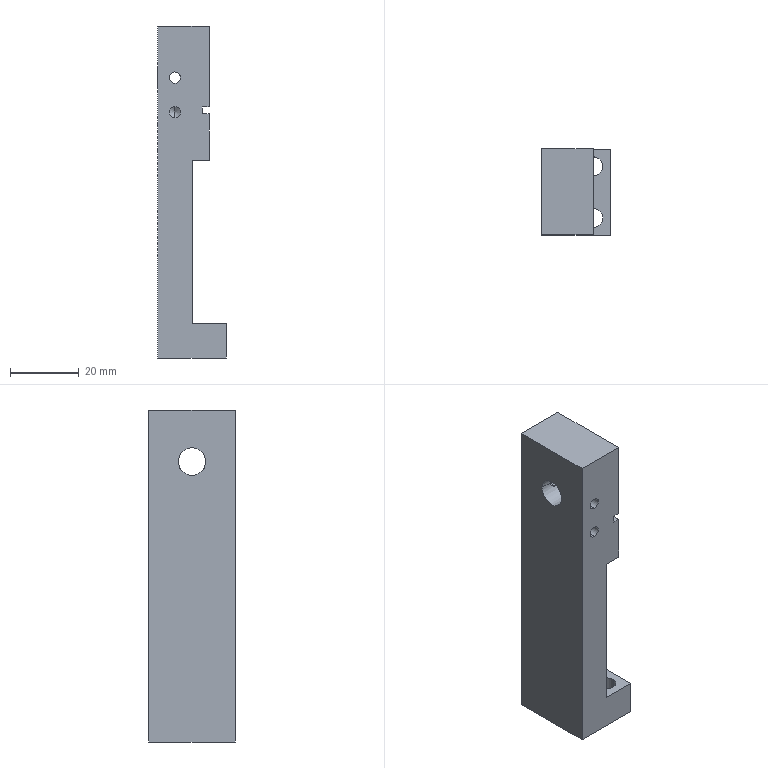Part | STEP file | 11-FG-B00211 | 1 solid | 40 faces | box 20 x 25 x 96.4 mm | volume 29627 mm3 | cylinder 18 | plane 14 | cone 8 | commonest cylinder face diameters 3.3 x12 5.5 x4 8 x2
STEP:
#1=CARTESIAN_POINT('',(4.,5.,71.65));
#2=VERTEX_POINT('',#1);
#3=CARTESIAN_POINT('',(4.,5.,68.35));
#4=VERTEX_POINT('',#3);
#5=CARTESIAN_POINT('',(4.,5.,70.));
#6=DIRECTION('',(1.,0.,0.));
#7=DIRECTION('',(0.,0.,-1.));
#8=AXIS2_PLACEMENT_3D('',#5,#6,#7);
#9=CIRCLE('',#8,1.65);
#10=EDGE_CURVE('',#2,#4,#9,.T.);
#11=ORIENTED_EDGE('',*,*,#10,.F.);
#12=CARTESIAN_POINT('',(15.,5.,71.65));
#13=VERTEX_POINT('',#12);
#14=CARTESIAN_POINT('',(15.,5.,71.65));
#15=DIRECTION('',(1.,0.,0.));
#16=VECTOR('',#15,1000.);
#17=LINE('',#14,#16);
#18=EDGE_CURVE('',#2,#13,#17,.T.);
#19=ORIENTED_EDGE('',*,*,#18,.T.);
#20=CARTESIAN_POINT('',(15.,5.,68.35));
#21=VERTEX_POINT('',#20);
#22=CARTESIAN_POINT('',(15.,5.,70.));
#23=DIRECTION('',(1.,0.,0.));
#24=DIRECTION('',(0.,0.,-1.));
#25=AXIS2_PLACEMENT_3D('',#22,#23,#24);
#26=CIRCLE('',#25,1.65);
#27=EDGE_CURVE('',#13,#21,#26,.T.);
#28=ORIENTED_EDGE('',*,*,#27,.T.);
#29=CARTESIAN_POINT('',(15.,5.,68.35));
#30=DIRECTION('',(1.,0.,0.));
#31=VECTOR('',#30,1000.);
#32=LINE('',#29,#31);
#33=EDGE_CURVE('',#4,#21,#32,.T.);
#34=ORIENTED_EDGE('',*,*,#33,.F.);
#35=EDGE_LOOP('',(#11,#19,#28,#34));
#36=FACE_OUTER_BOUND('',#35,.T.);
#37=CARTESIAN_POINT('',(15.,5.,70.));
#38=DIRECTION('',(1.,0.,0.));
#39=DIRECTION('',(0.,0.,-1.));
#40=AXIS2_PLACEMENT_3D('',#37,#38,#39);
#41=CYLINDRICAL_SURFACE('',#40,1.65);
#42=ADVANCED_FACE('',(#36),#41,.F.);
#43=CARTESIAN_POINT('',(3.009,5.,70.));
#44=VERTEX_POINT('',#43);
#45=CARTESIAN_POINT('',(4.,5.,68.35));
#46=DIRECTION('',(0.515,0.,-0.8572));
#47=VECTOR('',#46,1000.);
#48=LINE('',#45,#47);
#49=EDGE_CURVE('',#44,#4,#48,.T.);
#50=ORIENTED_EDGE('',*,*,#49,.F.);
#51=CARTESIAN_POINT('',(4.,5.,71.65));
#52=DIRECTION('',(0.515,0.,0.8572));
#53=VECTOR('',#52,1000.);
#54=LINE('',#51,#53);
#55=EDGE_CURVE('',#44,#2,#54,.T.);
#56=ORIENTED_EDGE('',*,*,#55,.T.);
#57=ORIENTED_EDGE('',*,*,#10,.T.);
#58=EDGE_LOOP('',(#50,#56,#57));
#59=FACE_OUTER_BOUND('',#58,.T.);
#60=CARTESIAN_POINT('',(4.,5.,70.));
#61=DIRECTION('',(1.,0.,0.));
#62=DIRECTION('',(0.,0.,-1.));
#63=AXIS2_PLACEMENT_3D('',#60,#61,#62);
#64=CONICAL_SURFACE('',#63,1.65,1.03);
#65=ADVANCED_FACE('',(#59),#64,.F.);
#66=CARTESIAN_POINT('',(4.,20.,71.65));
#67=VERTEX_POINT('',#66);
#68=CARTESIAN_POINT('',(4.,20.,68.35));
#69=VERTEX_POINT('',#68);
#70=CARTESIAN_POINT('',(4.,20.,70.));
#71=DIRECTION('',(1.,0.,0.));
#72=DIRECTION('',(0.,0.,-1.));
#73=AXIS2_PLACEMENT_3D('',#70,#71,#72);
#74=CIRCLE('',#73,1.65);
#75=EDGE_CURVE('',#67,#69,#74,.T.);
#76=ORIENTED_EDGE('',*,*,#75,.F.);
#77=CARTESIAN_POINT('',(15.,20.,71.65));
#78=VERTEX_POINT('',#77);
#79=CARTESIAN_POINT('',(15.,20.,71.65));
#80=DIRECTION('',(1.,0.,0.));
#81=VECTOR('',#80,1000.);
#82=LINE('',#79,#81);
#83=EDGE_CURVE('',#67,#78,#82,.T.);
#84=ORIENTED_EDGE('',*,*,#83,.T.);
#85=CARTESIAN_POINT('',(15.,20.,68.35));
#86=VERTEX_POINT('',#85);
#87=CARTESIAN_POINT('',(15.,20.,70.));
#88=DIRECTION('',(1.,0.,0.));
#89=DIRECTION('',(0.,0.,-1.));
#90=AXIS2_PLACEMENT_3D('',#87,#88,#89);
#91=CIRCLE('',#90,1.65);
#92=EDGE_CURVE('',#78,#86,#91,.T.);
#93=ORIENTED_EDGE('',*,*,#92,.T.);
#94=CARTESIAN_POINT('',(15.,20.,68.35));
#95=DIRECTION('',(1.,0.,0.));
#96=VECTOR('',#95,1000.);
#97=LINE('',#94,#96);
#98=EDGE_CURVE('',#69,#86,#97,.T.);
#99=ORIENTED_EDGE('',*,*,#98,.F.);
#100=EDGE_LOOP('',(#76,#84,#93,#99));
#101=FACE_OUTER_BOUND('',#100,.T.);
#102=CARTESIAN_POINT('',(15.,20.,70.));
#103=DIRECTION('',(1.,0.,0.));
#104=DIRECTION('',(0.,0.,-1.));
#105=AXIS2_PLACEMENT_3D('',#102,#103,#104);
#106=CYLINDRICAL_SURFACE('',#105,1.65);
#107=ADVANCED_FACE('',(#101),#106,.F.);
#108=CARTESIAN_POINT('',(3.009,20.,70.));
#109=VERTEX_POINT('',#108);
#110=CARTESIAN_POINT('',(4.,20.,68.35));
#111=DIRECTION('',(0.515,0.,-0.8572));
#112=VECTOR('',#111,1000.);
#113=LINE('',#110,#112);
#114=EDGE_CURVE('',#109,#69,#113,.T.);
#115=ORIENTED_EDGE('',*,*,#114,.F.);
#116=CARTESIAN_POINT('',(4.,20.,71.65));
#117=DIRECTION('',(0.515,0.,0.8572));
#118=VECTOR('',#117,1000.);
#119=LINE('',#116,#118);
#120=EDGE_CURVE('',#109,#67,#119,.T.);
#121=ORIENTED_EDGE('',*,*,#120,.T.);
#122=ORIENTED_EDGE('',*,*,#75,.T.);
#123=EDGE_LOOP('',(#115,#121,#122));
#124=FACE_OUTER_BOUND('',#123,.T.);
#125=CARTESIAN_POINT('',(4.,20.,70.));
#126=DIRECTION('',(1.,0.,0.));
#127=DIRECTION('',(0.,0.,-1.));
#128=AXIS2_PLACEMENT_3D('',#125,#126,#127);
#129=CONICAL_SURFACE('',#128,1.65,1.03);
#130=ADVANCED_FACE('',(#124),#129,.F.);
#131=CARTESIAN_POINT('',(5.,10.1,65.65));
#132=VERTEX_POINT('',#131);
#133=CARTESIAN_POINT('',(5.,10.1,62.35));
#134=VERTEX_POINT('',#133);
#135=CARTESIAN_POINT('',(5.,10.1,64.));
#136=DIRECTION('',(0.,-1.,0.));
#137=DIRECTION('',(0.,0.,-1.));
#138=AXIS2_PLACEMENT_3D('',#135,#136,#137);
#139=CIRCLE('',#138,1.65);
#140=EDGE_CURVE('',#132,#134,#139,.T.);
#141=ORIENTED_EDGE('',*,*,#140,.F.);
#142=CARTESIAN_POINT('',(5.,0.,65.65));
#143=VERTEX_POINT('',#142);
#144=CARTESIAN_POINT('',(5.,0.,65.65));
#145=DIRECTION('',(0.,-1.,0.));
#146=VECTOR('',#145,1000.);
#147=LINE('',#144,#146);
#148=EDGE_CURVE('',#132,#143,#147,.T.);
#149=ORIENTED_EDGE('',*,*,#148,.T.);
#150=CARTESIAN_POINT('',(5.,0.,62.35));
#151=VERTEX_POINT('',#150);
#152=CARTESIAN_POINT('',(5.,0.,64.));
#153=DIRECTION('',(0.,-1.,0.));
#154=DIRECTION('',(0.,0.,-1.));
#155=AXIS2_PLACEMENT_3D('',#152,#153,#154);
#156=CIRCLE('',#155,1.65);
#157=EDGE_CURVE('',#143,#151,#156,.T.);
#158=ORIENTED_EDGE('',*,*,#157,.T.);
#159=CARTESIAN_POINT('',(5.,0.,62.35));
#160=DIRECTION('',(0.,-1.,0.));
#161=VECTOR('',#160,1000.);
#162=LINE('',#159,#161);
#163=EDGE_CURVE('',#134,#151,#162,.T.);
#164=ORIENTED_EDGE('',*,*,#163,.F.);
#165=EDGE_LOOP('',(#141,#149,#158,#164));
#166=FACE_OUTER_BOUND('',#165,.T.);
#167=CARTESIAN_POINT('',(5.,0.,64.));
#168=DIRECTION('',(0.,-1.,0.));
#169=DIRECTION('',(0.,0.,-1.));
#170=AXIS2_PLACEMENT_3D('',#167,#168,#169);
#171=CYLINDRICAL_SURFACE('',#170,1.65);
#172=ADVANCED_FACE('',(#166),#171,.F.);
#173=CARTESIAN_POINT('',(5.,11.091,64.));
#174=VERTEX_POINT('',#173);
#175=CARTESIAN_POINT('',(5.,10.1,62.35));
#176=DIRECTION('',(0.,-0.515,-0.8572));
#177=VECTOR('',#176,1000.);
#178=LINE('',#175,#177);
#179=EDGE_CURVE('',#174,#134,#178,.T.);
#180=ORIENTED_EDGE('',*,*,#179,.F.);
#181=CARTESIAN_POINT('',(5.,10.1,65.65));
#182=DIRECTION('',(0.,-0.515,0.8572));
#183=VECTOR('',#182,1000.);
#184=LINE('',#181,#183);
#185=EDGE_CURVE('',#174,#132,#184,.T.);
#186=ORIENTED_EDGE('',*,*,#185,.T.);
#187=ORIENTED_EDGE('',*,*,#140,.T.);
#188=EDGE_LOOP('',(#180,#186,#187));
#189=FACE_OUTER_BOUND('',#188,.T.);
#190=CARTESIAN_POINT('',(5.,10.1,64.));
#191=DIRECTION('',(0.,-1.,0.));
#192=DIRECTION('',(0.,0.,-1.));
#193=AXIS2_PLACEMENT_3D('',#190,#191,#192);
#194=CONICAL_SURFACE('',#193,1.65,1.03);
#195=ADVANCED_FACE('',(#189),#194,.F.);
#196=CARTESIAN_POINT('',(5.,8.856,75.65));
#197=VERTEX_POINT('',#196);
#198=CARTESIAN_POINT('',(3.35,8.5,74.));
#199=VERTEX_POINT('',#198);
#200=CARTESIAN_POINT('',(5.,8.856,75.65));
#201=CARTESIAN_POINT('',(4.891,8.856,75.65));
#202=CARTESIAN_POINT('',(4.78,8.851,75.639));
#203=CARTESIAN_POINT('',(4.568,8.832,75.596));
#204=CARTESIAN_POINT('',(4.464,8.818,75.564));
#205=CARTESIAN_POINT('',(4.263,8.784,75.48));
#206=CARTESIAN_POINT('',(4.169,8.764,75.429));
#207=CARTESIAN_POINT('',(3.992,8.72,75.31));
#208=CARTESIAN_POINT('',(3.908,8.697,75.241));
#209=CARTESIAN_POINT('',(3.757,8.651,75.091));
#210=CARTESIAN_POINT('',(3.69,8.628,75.008));
#211=CARTESIAN_POINT('',(3.57,8.586,74.83));
#212=CARTESIAN_POINT('',(3.518,8.567,74.734));
#213=CARTESIAN_POINT('',(3.394,8.519,74.437));
#214=CARTESIAN_POINT('',(3.35,8.5,74.217));
#215=CARTESIAN_POINT('',(3.35,8.5,74.));
#216=B_SPLINE_CURVE_WITH_KNOTS('',3,(#200,#201,#202,#203,#204,#205,#206,#207,#208,#209,#210,#211,#212,#213,#214,#215),.UNSPECIFIED.,.F.,.F.,(4,2,2,2,2,2,2,4),(0.00261,0.002936,0.003262,0.003588,0.003914,0.00424,0.004566,0.005218),.UNSPECIFIED.);
#217=EDGE_CURVE('',#197,#199,#216,.T.);
#218=ORIENTED_EDGE('',*,*,#217,.F.);
#219=CARTESIAN_POINT('',(5.,0.,75.65));
#220=VERTEX_POINT('',#219);
#221=CARTESIAN_POINT('',(5.,0.,75.65));
#222=DIRECTION('',(0.,-1.,0.));
#223=VECTOR('',#222,1000.);
#224=LINE('',#221,#223);
#225=EDGE_CURVE('',#197,#220,#224,.T.);
#226=ORIENTED_EDGE('',*,*,#225,.T.);
#227=CARTESIAN_POINT('',(5.,0.,72.35));
#228=VERTEX_POINT('',#227);
#229=CARTESIAN_POINT('',(5.,0.,74.));
#230=DIRECTION('',(0.,-1.,0.));
#231=DIRECTION('',(0.,0.,-1.));
#232=AXIS2_PLACEMENT_3D('',#229,#230,#231);
#233=CIRCLE('',#232,1.65);
#234=EDGE_CURVE('',#220,#228,#233,.T.);
#235=ORIENTED_EDGE('',*,*,#234,.T.);
#236=CARTESIAN_POINT('',(5.,8.856,72.35));
#237=VERTEX_POINT('',#236);
#238=CARTESIAN_POINT('',(5.,0.,72.35));
#239=DIRECTION('',(0.,-1.,0.));
#240=VECTOR('',#239,1000.);
#241=LINE('',#238,#240);
#242=EDGE_CURVE('',#237,#228,#241,.T.);
#243=ORIENTED_EDGE('',*,*,#242,.F.);
#244=CARTESIAN_POINT('',(3.35,8.5,74.));
#245=CARTESIAN_POINT('',(3.35,8.5,73.891));
#246=CARTESIAN_POINT('',(3.361,8.505,73.781));
#247=CARTESIAN_POINT('',(3.404,8.522,73.567));
#248=CARTESIAN_POINT('',(3.436,8.535,73.464));
#249=CARTESIAN_POINT('',(3.561,8.583,73.164));
#250=CARTESIAN_POINT('',(3.682,8.628,72.984));
#251=CARTESIAN_POINT('',(3.91,8.697,72.756));
#252=CARTESIAN_POINT('',(3.993,8.72,72.689));
#253=CARTESIAN_POINT('',(4.17,8.764,72.57));
#254=CARTESIAN_POINT('',(4.266,8.784,72.518));
#255=CARTESIAN_POINT('',(4.465,8.818,72.435));
#256=CARTESIAN_POINT('',(4.568,8.832,72.404));
#257=CARTESIAN_POINT('',(4.781,8.851,72.361));
#258=CARTESIAN_POINT('',(4.891,8.856,72.35));
#259=CARTESIAN_POINT('',(5.,8.856,72.35));
#260=B_SPLINE_CURVE_WITH_KNOTS('',3,(#244,#245,#246,#247,#248,#249,#250,#251,#252,#253,#254,#255,#256,#257,#258,#259),.UNSPECIFIED.,.F.,.F.,(4,2,2,2,2,2,2,4),(0.005218,0.005543,0.005869,0.006521,0.006847,0.007173,0.007499,0.007825),.UNSPECIFIED.);
#261=EDGE_CURVE('',#199,#237,#260,.T.);
#262=ORIENTED_EDGE('',*,*,#261,.F.);
#263=EDGE_LOOP('',(#218,#226,#235,#243,#262));
#264=FACE_OUTER_BOUND('',#263,.T.);
#265=CARTESIAN_POINT('',(5.,0.,74.));
#266=DIRECTION('',(0.,-1.,0.));
#267=DIRECTION('',(0.,0.,-1.));
#268=AXIS2_PLACEMENT_3D('',#265,#266,#267);
#269=CYLINDRICAL_SURFACE('',#268,1.65);
#270=ADVANCED_FACE('',(#264),#269,.F.);
#271=CARTESIAN_POINT('',(12.25,5.,-7.4));
#272=VERTEX_POINT('',#271);
#273=CARTESIAN_POINT('',(17.75,5.,-7.4));
#274=VERTEX_POINT('',#273);
#275=CARTESIAN_POINT('',(15.,5.,-7.4));
#276=DIRECTION('',(0.,0.,1.));
#277=DIRECTION('',(1.,0.,0.));
#278=AXIS2_PLACEMENT_3D('',#275,#276,#277);
#279=CIRCLE('',#278,2.75);
#280=EDGE_CURVE('',#272,#274,#279,.T.);
#281=ORIENTED_EDGE('',*,*,#280,.F.);
#282=CARTESIAN_POINT('',(12.25,5.,2.6));
#283=VERTEX_POINT('',#282);
#284=CARTESIAN_POINT('',(12.25,5.,0.));
#285=DIRECTION('',(0.,0.,1.));
#286=VECTOR('',#285,1000.);
#287=LINE('',#284,#286);
#288=EDGE_CURVE('',#272,#283,#287,.T.);
#289=ORIENTED_EDGE('',*,*,#288,.T.);
#290=CARTESIAN_POINT('',(17.75,5.,2.6));
#291=VERTEX_POINT('',#290);
#292=CARTESIAN_POINT('',(15.,5.,2.6));
#293=DIRECTION('',(0.,0.,1.));
#294=DIRECTION('',(1.,0.,0.));
#295=AXIS2_PLACEMENT_3D('',#292,#293,#294);
#296=CIRCLE('',#295,2.75);
#297=EDGE_CURVE('',#283,#291,#296,.T.);
#298=ORIENTED_EDGE('',*,*,#297,.T.);
#299=CARTESIAN_POINT('',(17.75,5.,0.));
#300=DIRECTION('',(0.,0.,1.));
#301=VECTOR('',#300,1000.);
#302=LINE('',#299,#301);
#303=EDGE_CURVE('',#274,#291,#302,.T.);
#304=ORIENTED_EDGE('',*,*,#303,.F.);
#305=EDGE_LOOP('',(#281,#289,#298,#304));
#306=FACE_OUTER_BOUND('',#305,.T.);
#307=CARTESIAN_POINT('',(15.,5.,0.));
#308=DIRECTION('',(0.,0.,1.));
#309=DIRECTION('',(1.,0.,0.));
#310=AXIS2_PLACEMENT_3D('',#307,#308,#309);
#311=CYLINDRICAL_SURFACE('',#310,2.75);
#312=ADVANCED_FACE('',(#306),#311,.F.);
#313=CARTESIAN_POINT('',(12.25,20.,-7.4));
#314=VERTEX_POINT('',#313);
#315=CARTESIAN_POINT('',(17.75,20.,-7.4));
#316=VERTEX_POINT('',#315);
#317=CARTESIAN_POINT('',(15.,20.,-7.4));
#318=DIRECTION('',(0.,0.,1.));
#319=DIRECTION('',(1.,0.,0.));
#320=AXIS2_PLACEMENT_3D('',#317,#318,#319);
#321=CIRCLE('',#320,2.75);
#322=EDGE_CURVE('',#314,#316,#321,.T.);
#323=ORIENTED_EDGE('',*,*,#322,.F.);
#324=CARTESIAN_POINT('',(12.25,20.,2.6));
#325=VERTEX_POINT('',#324);
#326=CARTESIAN_POINT('',(12.25,20.,0.));
#327=DIRECTION('',(0.,0.,1.));
#328=VECTOR('',#327,1000.);
#329=LINE('',#326,#328);
#330=EDGE_CURVE('',#314,#325,#329,.T.);
#331=ORIENTED_EDGE('',*,*,#330,.T.);
#332=CARTESIAN_POINT('',(17.75,20.,2.6));
#333=VERTEX_POINT('',#332);
#334=CARTESIAN_POINT('',(15.,20.,2.6));
#335=DIRECTION('',(0.,0.,1.));
#336=DIRECTION('',(1.,0.,0.));
#337=AXIS2_PLACEMENT_3D('',#334,#335,#336);
#338=CIRCLE('',#337,2.75);
#339=EDGE_CURVE('',#325,#333,#338,.T.);
#340=ORIENTED_EDGE('',*,*,#339,.T.);
#341=CARTESIAN_POINT('',(17.75,20.,0.));
#342=DIRECTION('',(0.,0.,1.));
#343=VECTOR('',#342,1000.);
#344=LINE('',#341,#343);
#345=EDGE_CURVE('',#316,#333,#344,.T.);
#346=ORIENTED_EDGE('',*,*,#345,.F.);
#347=EDGE_LOOP('',(#323,#331,#340,#346));
#348=FACE_OUTER_BOUND('',#347,.T.);
#349=CARTESIAN_POINT('',(15.,20.,0.));
#350=DIRECTION('',(0.,0.,1.));
#351=DIRECTION('',(1.,0.,0.));
#352=AXIS2_PLACEMENT_3D('',#349,#350,#351);
#353=CYLINDRICAL_SURFACE('',#352,2.75);
#354=ADVANCED_FACE('',(#348),#353,.F.);
#355=CARTESIAN_POINT('',(5.,16.144,72.35));
#356=VERTEX_POINT('',#355);
#357=CARTESIAN_POINT('',(3.35,16.5,74.));
#358=VERTEX_POINT('',#357);
#359=CARTESIAN_POINT('',(5.,16.144,72.35));
#360=CARTESIAN_POINT('',(4.891,16.144,72.35));
#361=CARTESIAN_POINT('',(4.781,16.149,72.361));
#362=CARTESIAN_POINT('',(4.568,16.168,72.404));
#363=CARTESIAN_POINT('',(4.464,16.182,72.436));
#364=CARTESIAN_POINT('',(4.165,16.233,72.561));
#365=CARTESIAN_POINT('',(3.985,16.28,72.682));
#366=CARTESIAN_POINT('',(3.757,16.349,72.91));
#367=CARTESIAN_POINT('',(3.689,16.372,72.992));
#368=CARTESIAN_POINT('',(3.571,16.414,73.169));
#369=CARTESIAN_POINT('',(3.519,16.433,73.265));
#370=CARTESIAN_POINT('',(3.436,16.465,73.465));
#371=CARTESIAN_POINT('',(3.404,16.478,73.568));
#372=CARTESIAN_POINT('',(3.361,16.495,73.781));
#373=CARTESIAN_POINT('',(3.35,16.5,73.891));
#374=CARTESIAN_POINT('',(3.35,16.5,74.));
#375=B_SPLINE_CURVE_WITH_KNOTS('',3,(#359,#360,#361,#362,#363,#364,#365,#366,#367,#368,#369,#370,#371,#372,#373,#374),.UNSPECIFIED.,.F.,.F.,(4,2,2,2,2,2,2,4),(0.005217,0.005543,0.005869,0.006521,0.006847,0.007172,0.007498,0.007824),.UNSPECIFIED.);
#376=EDGE_CURVE('',#356,#358,#375,.T.);
#377=ORIENTED_EDGE('',*,*,#376,.F.);
#378=CARTESIAN_POINT('',(5.,25.,72.35));
#379=VERTEX_POINT('',#378);
#380=CARTESIAN_POINT('',(5.,25.,72.35));
#381=DIRECTION('',(0.,1.,0.));
#382=VECTOR('',#381,1000.);
#383=LINE('',#380,#382);
#384=EDGE_CURVE('',#356,#379,#383,.T.);
#385=ORIENTED_EDGE('',*,*,#384,.T.);
#386=CARTESIAN_POINT('',(5.,25.,75.65));
#387=VERTEX_POINT('',#386);
#388=CARTESIAN_POINT('',(5.,25.,74.));
#389=DIRECTION('',(0.,1.,0.));
#390=DIRECTION('',(0.,0.,1.));
#391=AXIS2_PLACEMENT_3D('',#388,#389,#390);
#392=CIRCLE('',#391,1.65);
#393=EDGE_CURVE('',#379,#387,#392,.T.);
#394=ORIENTED_EDGE('',*,*,#393,.T.);
#395=CARTESIAN_POINT('',(5.,16.144,75.65));
#396=VERTEX_POINT('',#395);
#397=CARTESIAN_POINT('',(5.,25.,75.65));
#398=DIRECTION('',(0.,1.,0.));
#399=VECTOR('',#398,1000.);
#400=LINE('',#397,#399);
#401=EDGE_CURVE('',#396,#387,#400,.T.);
#402=ORIENTED_EDGE('',*,*,#401,.F.);
#403=CARTESIAN_POINT('',(3.35,16.5,74.));
#404=CARTESIAN_POINT('',(3.35,16.5,74.218));
#405=CARTESIAN_POINT('',(3.394,16.481,74.437));
#406=CARTESIAN_POINT('',(3.519,16.433,74.735));
#407=CARTESIAN_POINT('',(3.571,16.414,74.831));
#408=CARTESIAN_POINT('',(3.69,16.372,75.009));
#409=CARTESIAN_POINT('',(3.758,16.349,75.091));
#410=CARTESIAN_POINT('',(3.909,16.303,75.243));
#411=CARTESIAN_POINT('',(3.993,16.279,75.311));
#412=CARTESIAN_POINT('',(4.17,16.236,75.43));
#413=CARTESIAN_POINT('',(4.264,16.216,75.481));
#414=CARTESIAN_POINT('',(4.565,16.164,75.607));
#415=CARTESIAN_POINT('',(4.779,16.144,75.65));
#416=CARTESIAN_POINT('',(5.,16.144,75.65));
#417=B_SPLINE_CURVE_WITH_KNOTS('',3,(#403,#404,#405,#406,#407,#408,#409,#410,#411,#412,#413,#414,#415,#416),.UNSPECIFIED.,.F.,.F.,(4,2,2,2,2,2,4),(0.007824,0.008476,0.008802,0.009127,0.009453,0.009779,0.01043),.UNSPECIFIED.);
#418=EDGE_CURVE('',#358,#396,#417,.T.);
#419=ORIENTED_EDGE('',*,*,#418,.F.);
#420=EDGE_LOOP('',(#377,#385,#394,#402,#419));
#421=FACE_OUTER_BOUND('',#420,.T.);
#422=CARTESIAN_POINT('',(5.,25.,74.));
#423=DIRECTION('',(0.,1.,0.));
#424=DIRECTION('',(0.,0.,1.));
#425=AXIS2_PLACEMENT_3D('',#422,#423,#424);
#426=CYLINDRICAL_SURFACE('',#425,1.65);
#427=ADVANCED_FACE('',(#421),#426,.F.);
#428=CARTESIAN_POINT('',(5.,14.9,62.35));
#429=VERTEX_POINT('',#428);
#430=CARTESIAN_POINT('',(5.,14.9,65.65));
#431=VERTEX_POINT('',#430);
#432=CARTESIAN_POINT('',(5.,14.9,64.));
#433=DIRECTION('',(0.,1.,0.));
#434=DIRECTION('',(0.,0.,1.));
#435=AXIS2_PLACEMENT_3D('',#432,#433,#434);
#436=CIRCLE('',#435,1.65);
#437=EDGE_CURVE('',#429,#431,#436,.T.);
#438=ORIENTED_EDGE('',*,*,#437,.F.);
#439=CARTESIAN_POINT('',(5.,25.,62.35));
#440=VERTEX_POINT('',#439);
#441=CARTESIAN_POINT('',(5.,25.,62.35));
#442=DIRECTION('',(0.,1.,0.));
#443=VECTOR('',#442,1000.);
#444=LINE('',#441,#443);
#445=EDGE_CURVE('',#429,#440,#444,.T.);
#446=ORIENTED_EDGE('',*,*,#445,.T.);
#447=CARTESIAN_POINT('',(5.,25.,65.65));
#448=VERTEX_POINT('',#447);
#449=CARTESIAN_POINT('',(5.,25.,64.));
#450=DIRECTION('',(0.,1.,0.));
#451=DIRECTION('',(0.,0.,1.));
#452=AXIS2_PLACEMENT_3D('',#449,#450,#451);
#453=CIRCLE('',#452,1.65);
#454=EDGE_CURVE('',#440,#448,#453,.T.);
#455=ORIENTED_EDGE('',*,*,#454,.T.);
#456=CARTESIAN_POINT('',(5.,25.,65.65));
#457=DIRECTION('',(0.,1.,0.));
#458=VECTOR('',#457,1000.);
#459=LINE('',#456,#458);
#460=EDGE_CURVE('',#431,#448,#459,.T.);
#461=ORIENTED_EDGE('',*,*,#460,.F.);
#462=EDGE_LOOP('',(#438,#446,#455,#461));
#463=FACE_OUTER_BOUND('',#462,.T.);
#464=CARTESIAN_POINT('',(5.,25.,64.));
#465=DIRECTION('',(0.,1.,0.));
#466=DIRECTION('',(0.,0.,1.));
#467=AXIS2_PLACEMENT_3D('',#464,#465,#466);
#468=CYLINDRICAL_SURFACE('',#467,1.65);
#469=ADVANCED_FACE('',(#463),#468,.F.);
#470=CARTESIAN_POINT('',(5.,13.909,64.));
#471=VERTEX_POINT('',#470);
#472=CARTESIAN_POINT('',(5.,14.9,65.65));
#473=DIRECTION('',(0.,0.515,0.8572));
#474=VECTOR('',#473,1000.);
#475=LINE('',#472,#474);
#476=EDGE_CURVE('',#471,#431,#475,.T.);
#477=ORIENTED_EDGE('',*,*,#476,.F.);
#478=CARTESIAN_POINT('',(5.,14.9,62.35));
#479=DIRECTION('',(0.,0.515,-0.8572));
#480=VECTOR('',#479,1000.);
#481=LINE('',#478,#480);
#482=EDGE_CURVE('',#471,#429,#481,.T.);
#483=ORIENTED_EDGE('',*,*,#482,.T.);
#484=ORIENTED_EDGE('',*,*,#437,.T.);
#485=EDGE_LOOP('',(#477,#483,#484));
#486=FACE_OUTER_BOUND('',#485,.T.);
#487=CARTESIAN_POINT('',(5.,14.9,64.));
#488=DIRECTION('',(0.,1.,0.));
#489=DIRECTION('',(0.,0.,1.));
#490=AXIS2_PLACEMENT_3D('',#487,#488,#489);
#491=CONICAL_SURFACE('',#490,1.65,1.03);
#492=ADVANCED_FACE('',(#486),#491,.F.);
#493=CARTESIAN_POINT('',(15.,16.5,74.));
#494=VERTEX_POINT('',#493);
#495=CARTESIAN_POINT('',(15.,8.5,74.));
#496=VERTEX_POINT('',#495);
#497=CARTESIAN_POINT('',(15.,12.5,74.));
#498=DIRECTION('',(-1.,0.,0.));
#499=DIRECTION('',(0.,-1.,0.));
#500=AXIS2_PLACEMENT_3D('',#497,#498,#499);
#501=CIRCLE('',#500,4.);
#502=EDGE_CURVE('',#494,#496,#501,.T.);
#503=ORIENTED_EDGE('',*,*,#502,.F.);
#504=CARTESIAN_POINT('',(6.65,16.5,74.));
#505=VERTEX_POINT('',#504);
#506=CARTESIAN_POINT('',(20.,16.5,74.));
#507=DIRECTION('',(-1.,0.,0.));
#508=VECTOR('',#507,1000.);
#509=LINE('',#506,#508);
#510=EDGE_CURVE('',#494,#505,#509,.T.);
#511=ORIENTED_EDGE('',*,*,#510,.T.);
#512=CARTESIAN_POINT('',(6.65,16.5,74.));
#513=CARTESIAN_POINT('',(6.65,16.5,73.891));
#514=CARTESIAN_POINT('',(6.639,16.495,73.78));
#515=CARTESIAN_POINT('',(6.596,16.478,73.568));
#516=CARTESIAN_POINT('',(6.564,16.465,73.464));
#517=CARTESIAN_POINT('',(6.48,16.433,73.263));
#518=CARTESIAN_POINT('',(6.429,16.414,73.168));
#519=CARTESIAN_POINT('',(6.31,16.372,72.991));
#520=CARTESIAN_POINT('',(6.241,16.349,72.907));
#521=CARTESIAN_POINT('',(6.09,16.303,72.756));
#522=CARTESIAN_POINT('',(6.008,16.28,72.689));
#523=CARTESIAN_POINT('',(5.829,16.236,72.57));
#524=CARTESIAN_POINT('',(5.734,16.216,72.518));
#525=CARTESIAN_POINT('',(5.437,16.165,72.394));
#526=CARTESIAN_POINT('',(5.217,16.144,72.35));
#527=CARTESIAN_POINT('',(5.,16.144,72.35));
#528=B_SPLINE_CURVE_WITH_KNOTS('',3,(#512,#513,#514,#515,#516,#517,#518,#519,#520,#521,#522,#523,#524,#525,#526,#527),.UNSPECIFIED.,.F.,.F.,(4,2,2,2,2,2,2,4),(0.00261,0.002935,0.003261,0.003587,0.003913,0.004239,0.004565,0.005217),.UNSPECIFIED.);
#529=EDGE_CURVE('',#505,#356,#528,.T.);
#530=ORIENTED_EDGE('',*,*,#529,.T.);
#531=ORIENTED_EDGE('',*,*,#376,.T.);
#532=CARTESIAN_POINT('',(0.,16.5,74.));
#533=VERTEX_POINT('',#532);
#534=CARTESIAN_POINT('',(20.,16.5,74.));
#535=DIRECTION('',(-1.,0.,0.));
#536=VECTOR('',#535,1000.);
#537=LINE('',#534,#536);
#538=EDGE_CURVE('',#358,#533,#537,.T.);
#539=ORIENTED_EDGE('',*,*,#538,.T.);
#540=CARTESIAN_POINT('',(0.,8.5,74.));
#541=VERTEX_POINT('',#540);
#542=CARTESIAN_POINT('',(0.,12.5,74.));
#543=DIRECTION('',(-1.,0.,0.));
#544=DIRECTION('',(0.,-1.,0.));
#545=AXIS2_PLACEMENT_3D('',#542,#543,#544);
#546=CIRCLE('',#545,4.);
#547=EDGE_CURVE('',#533,#541,#546,.T.);
#548=ORIENTED_EDGE('',*,*,#547,.T.);
#549=CARTESIAN_POINT('',(20.,8.5,74.));
#550=DIRECTION('',(-1.,0.,0.));
#551=VECTOR('',#550,1000.);
#552=LINE('',#549,#551);
#553=EDGE_CURVE('',#199,#541,#552,.T.);
#554=ORIENTED_EDGE('',*,*,#553,.F.);
#555=ORIENTED_EDGE('',*,*,#261,.T.);
#556=CARTESIAN_POINT('',(6.65,8.5,74.));
#557=VERTEX_POINT('',#556);
#558=CARTESIAN_POINT('',(5.,8.856,72.35));
#559=CARTESIAN_POINT('',(5.217,8.856,72.35));
#560=CARTESIAN_POINT('',(5.436,8.835,72.394));
#561=CARTESIAN_POINT('',(5.734,8.784,72.519));
#562=CARTESIAN_POINT('',(5.831,8.764,72.57));
#563=CARTESIAN_POINT('',(6.008,8.72,72.69));
#564=CARTESIAN_POINT('',(6.09,8.697,72.757));
#565=CARTESIAN_POINT('',(6.242,8.651,72.908));
#566=CARTESIAN_POINT('',(6.311,8.628,72.992));
#567=CARTESIAN_POINT('',(6.429,8.586,73.169));
#568=CARTESIAN_POINT('',(6.48,8.567,73.263));
#569=CARTESIAN_POINT('',(6.607,8.518,73.565));
#570=CARTESIAN_POINT('',(6.65,8.5,73.78));
#571=CARTESIAN_POINT('',(6.65,8.5,74.));
#572=B_SPLINE_CURVE_WITH_KNOTS('',3,(#558,#559,#560,#561,#562,#563,#564,#565,#566,#567,#568,#569,#570,#571),.UNSPECIFIED.,.F.,.F.,(4,2,2,2,2,2,4),(0.007825,0.008476,0.008802,0.009128,0.009454,0.00978,0.01043),.UNSPECIFIED.);
#573=EDGE_CURVE('',#237,#557,#572,.T.);
#574=ORIENTED_EDGE('',*,*,#573,.T.);
#575=CARTESIAN_POINT('',(20.,8.5,74.));
#576=DIRECTION('',(-1.,0.,0.));
#577=VECTOR('',#576,1000.);
#578=LINE('',#575,#577);
#579=EDGE_CURVE('',#496,#557,#578,.T.);
#580=ORIENTED_EDGE('',*,*,#579,.F.);
#581=EDGE_LOOP('',(#503,#511,#530,#531,#539,#548,#554,#555,#574,#580));
#582=FACE_OUTER_BOUND('',#581,.T.);
#583=CARTESIAN_POINT('',(20.,12.5,74.));
#584=DIRECTION('',(-1.,0.,0.));
#585=DIRECTION('',(0.,-1.,0.));
#586=AXIS2_PLACEMENT_3D('',#583,#584,#585);
#587=CYLINDRICAL_SURFACE('',#586,4.);
#588=ADVANCED_FACE('',(#582),#587,.F.);
#589=CARTESIAN_POINT('',(15.,12.5,74.));
#590=DIRECTION('',(-1.,0.,0.));
#591=DIRECTION('',(0.,-1.,0.));
#592=AXIS2_PLACEMENT_3D('',#589,#590,#591);
#593=CIRCLE('',#592,4.);
#594=EDGE_CURVE('',#496,#494,#593,.T.);
#595=ORIENTED_EDGE('',*,*,#594,.T.);
#596=ORIENTED_EDGE('',*,*,#502,.T.);
#597=EDGE_LOOP('',(#595,#596));
#598=FACE_BOUND('',#597,.T.);
#599=CARTESIAN_POINT('',(15.,20.,70.));
#600=DIRECTION('',(1.,0.,0.));
#601=DIRECTION('',(0.,0.,-1.));
#602=AXIS2_PLACEMENT_3D('',#599,#600,#601);
#603=CIRCLE('',#602,1.65);
#604=EDGE_CURVE('',#86,#78,#603,.T.);
#605=ORIENTED_EDGE('',*,*,#604,.F.);
#606=ORIENTED_EDGE('',*,*,#92,.F.);
#607=EDGE_LOOP('',(#605,#606));
#608=FACE_BOUND('',#607,.T.);
#609=CARTESIAN_POINT('',(15.,5.,70.));
#610=DIRECTION('',(1.,0.,0.));
#611=DIRECTION('',(0.,0.,-1.));
#612=AXIS2_PLACEMENT_3D('',#609,#610,#611);
#613=CIRCLE('',#612,1.65);
#614=EDGE_CURVE('',#21,#13,#613,.T.);
#615=ORIENTED_EDGE('',*,*,#614,.F.);
#616=ORIENTED_EDGE('',*,*,#27,.F.);
#617=EDGE_LOOP('',(#615,#616));
#618=FACE_BOUND('',#617,.T.);
#619=CARTESIAN_POINT('',(15.,0.,89.));
#620=VERTEX_POINT('',#619);
#621=CARTESIAN_POINT('',(15.,0.,65.5));
#622=VERTEX_POINT('',#621);
#623=CARTESIAN_POINT('',(15.,0.,89.));
#624=DIRECTION('',(0.,0.,-1.));
#625=VECTOR('',#624,1000.);
#626=LINE('',#623,#625);
#627=EDGE_CURVE('',#620,#622,#626,.T.);
#628=ORIENTED_EDGE('',*,*,#627,.T.);
#629=CARTESIAN_POINT('',(15.,25.,65.5));
#630=VERTEX_POINT('',#629);
#631=CARTESIAN_POINT('',(15.,-22.,65.5));
#632=DIRECTION('',(0.,1.,0.));
#633=VECTOR('',#632,1000.);
#634=LINE('',#631,#633);
#635=EDGE_CURVE('',#622,#630,#634,.T.);
#636=ORIENTED_EDGE('',*,*,#635,.T.);
#637=CARTESIAN_POINT('',(15.,25.,89.));
#638=VERTEX_POINT('',#637);
#639=CARTESIAN_POINT('',(15.,25.,89.));
#640=DIRECTION('',(0.,0.,-1.));
#641=VECTOR('',#640,1000.);
#642=LINE('',#639,#641);
#643=EDGE_CURVE('',#638,#630,#642,.T.);
#644=ORIENTED_EDGE('',*,*,#643,.F.);
#645=CARTESIAN_POINT('',(15.,0.,89.));
#646=DIRECTION('',(0.,1.,0.));
#647=VECTOR('',#646,1000.);
#648=LINE('',#645,#647);
#649=EDGE_CURVE('',#620,#638,#648,.T.);
#650=ORIENTED_EDGE('',*,*,#649,.F.);
#651=EDGE_LOOP('',(#628,#636,#644,#650));
#652=FACE_OUTER_BOUND('',#651,.T.);
#653=CARTESIAN_POINT('',(15.,0.,89.));
#654=DIRECTION('',(-1.,0.,0.));
#655=DIRECTION('',(0.,-1.,0.));
#656=AXIS2_PLACEMENT_3D('',#653,#654,#655);
#657=PLANE('',#656);
#658=ADVANCED_FACE('',(#598,#608,#618,#652),#657,.F.);
#659=CARTESIAN_POINT('',(0.,12.5,74.));
#660=DIRECTION('',(-1.,0.,0.));
#661=DIRECTION('',(0.,-1.,0.));
#662=AXIS2_PLACEMENT_3D('',#659,#660,#661);
#663=CIRCLE('',#662,4.);
#664=EDGE_CURVE('',#541,#533,#663,.T.);
#665=ORIENTED_EDGE('',*,*,#664,.F.);
#666=ORIENTED_EDGE('',*,*,#547,.F.);
#667=EDGE_LOOP('',(#665,#666));
#668=FACE_BOUND('',#667,.T.);
#669=CARTESIAN_POINT('',(0.,25.,-7.4));
#670=VERTEX_POINT('',#669);
#671=CARTESIAN_POINT('',(0.,0.,-7.4));
#672=VERTEX_POINT('',#671);
#673=CARTESIAN_POINT('',(0.,0.,-7.4));
#674=DIRECTION('',(0.,-1.,0.));
#675=VECTOR('',#674,1000.);
#676=LINE('',#673,#675);
#677=EDGE_CURVE('',#670,#672,#676,.T.);
#678=ORIENTED_EDGE('',*,*,#677,.T.);
#679=CARTESIAN_POINT('',(0.,0.,89.));
#680=VERTEX_POINT('',#679);
#681=CARTESIAN_POINT('',(0.,0.,89.));
#682=DIRECTION('',(0.,0.,-1.));
#683=VECTOR('',#682,1000.);
#684=LINE('',#681,#683);
#685=EDGE_CURVE('',#680,#672,#684,.T.);
#686=ORIENTED_EDGE('',*,*,#685,.F.);
#687=CARTESIAN_POINT('',(0.,25.,89.));
#688=VERTEX_POINT('',#687);
#689=CARTESIAN_POINT('',(0.,0.,89.));
#690=DIRECTION('',(0.,-1.,0.));
#691=VECTOR('',#690,1000.);
#692=LINE('',#689,#691);
#693=EDGE_CURVE('',#688,#680,#692,.T.);
#694=ORIENTED_EDGE('',*,*,#693,.F.);
#695=CARTESIAN_POINT('',(0.,25.,89.));
#696=DIRECTION('',(0.,0.,-1.));
#697=VECTOR('',#696,1000.);
#698=LINE('',#695,#697);
#699=EDGE_CURVE('',#688,#670,#698,.T.);
#700=ORIENTED_EDGE('',*,*,#699,.T.);
#701=EDGE_LOOP('',(#678,#686,#694,#700));
#702=FACE_OUTER_BOUND('',#701,.T.);
#703=CARTESIAN_POINT('',(0.,0.,89.));
#704=DIRECTION('',(1.,0.,0.));
#705=DIRECTION('',(0.,1.,0.));
#706=AXIS2_PLACEMENT_3D('',#703,#704,#705);
#707=PLANE('',#706);
#708=ADVANCED_FACE('',(#668,#702),#707,.F.);
#709=CARTESIAN_POINT('',(5.,0.,64.));
#710=DIRECTION('',(0.,-1.,0.));
#711=DIRECTION('',(0.,0.,-1.));
#712=AXIS2_PLACEMENT_3D('',#709,#710,#711);
#713=CIRCLE('',#712,1.65);
#714=EDGE_CURVE('',#151,#143,#713,.T.);
#715=ORIENTED_EDGE('',*,*,#714,.F.);
#716=ORIENTED_EDGE('',*,*,#157,.F.);
#717=EDGE_LOOP('',(#715,#716));
#718=FACE_BOUND('',#717,.T.);
#719=CARTESIAN_POINT('',(5.,0.,74.));
#720=DIRECTION('',(0.,-1.,0.));
#721=DIRECTION('',(0.,0.,-1.));
#722=AXIS2_PLACEMENT_3D('',#719,#720,#721);
#723=CIRCLE('',#722,1.65);
#724=EDGE_CURVE('',#228,#220,#723,.T.);
#725=ORIENTED_EDGE('',*,*,#724,.F.);
#726=ORIENTED_EDGE('',*,*,#234,.F.);
#727=EDGE_LOOP('',(#725,#726));
#728=FACE_BOUND('',#727,.T.);
#729=CARTESIAN_POINT('',(13.,0.,63.5));
#730=VERTEX_POINT('',#729);
#731=CARTESIAN_POINT('',(13.,0.,65.5));
#732=VERTEX_POINT('',#731);
#733=CARTESIAN_POINT('',(13.,0.,89.));
#734=DIRECTION('',(0.,0.,1.));
#735=VECTOR('',#734,1000.);
#736=LINE('',#733,#735);
#737=EDGE_CURVE('',#730,#732,#736,.T.);
#738=ORIENTED_EDGE('',*,*,#737,.T.);
#739=CARTESIAN_POINT('',(0.,0.,65.5));
#740=DIRECTION('',(1.,0.,0.));
#741=VECTOR('',#740,1000.);
#742=LINE('',#739,#741);
#743=EDGE_CURVE('',#732,#622,#742,.T.);
#744=ORIENTED_EDGE('',*,*,#743,.T.);
#745=ORIENTED_EDGE('',*,*,#627,.F.);
#746=CARTESIAN_POINT('',(0.,0.,89.));
#747=DIRECTION('',(1.,0.,0.));
#748=VECTOR('',#747,1000.);
#749=LINE('',#746,#748);
#750=EDGE_CURVE('',#680,#620,#749,.T.);
#751=ORIENTED_EDGE('',*,*,#750,.F.);
#752=ORIENTED_EDGE('',*,*,#685,.T.);
#753=CARTESIAN_POINT('',(20.,0.,-7.4));
#754=VERTEX_POINT('',#753);
#755=CARTESIAN_POINT('',(0.,0.,-7.4));
#756=DIRECTION('',(1.,0.,0.));
#757=VECTOR('',#756,1000.);
#758=LINE('',#755,#757);
#759=EDGE_CURVE('',#672,#754,#758,.T.);
#760=ORIENTED_EDGE('',*,*,#759,.T.);
#761=CARTESIAN_POINT('',(20.,0.,2.6));
#762=VERTEX_POINT('',#761);
#763=CARTESIAN_POINT('',(20.,0.,10.));
#764=DIRECTION('',(0.,0.,-1.));
#765=VECTOR('',#764,1000.);
#766=LINE('',#763,#765);
#767=EDGE_CURVE('',#762,#754,#766,.T.);
#768=ORIENTED_EDGE('',*,*,#767,.F.);
#769=CARTESIAN_POINT('',(10.,0.,2.6));
#770=VERTEX_POINT('',#769);
#771=CARTESIAN_POINT('',(15.,0.,2.6));
#772=DIRECTION('',(1.,0.,0.));
#773=VECTOR('',#772,1000.);
#774=LINE('',#771,#773);
#775=EDGE_CURVE('',#770,#762,#774,.T.);
#776=ORIENTED_EDGE('',*,*,#775,.F.);
#777=CARTESIAN_POINT('',(10.,0.,50.));
#778=VERTEX_POINT('',#777);
#779=CARTESIAN_POINT('',(10.,0.,10.));
#780=DIRECTION('',(0.,0.,-1.));
#781=VECTOR('',#780,1000.);
#782=LINE('',#779,#781);
#783=EDGE_CURVE('',#778,#770,#782,.T.);
#784=ORIENTED_EDGE('',*,*,#783,.F.);
#785=CARTESIAN_POINT('',(15.,0.,50.));
#786=VERTEX_POINT('',#785);
#787=CARTESIAN_POINT('',(15.,0.,50.));
#788=DIRECTION('',(-1.,0.,0.));
#789=VECTOR('',#788,1000.);
#790=LINE('',#787,#789);
#791=EDGE_CURVE('',#786,#778,#790,.T.);
#792=ORIENTED_EDGE('',*,*,#791,.F.);
#793=CARTESIAN_POINT('',(15.,0.,63.5));
#794=VERTEX_POINT('',#793);
#795=CARTESIAN_POINT('',(15.,0.,89.));
#796=DIRECTION('',(0.,0.,-1.));
#797=VECTOR('',#796,1000.);
#798=LINE('',#795,#797);
#799=EDGE_CURVE('',#794,#786,#798,.T.);
#800=ORIENTED_EDGE('',*,*,#799,.F.);
#801=CARTESIAN_POINT('',(0.,0.,63.5));
#802=DIRECTION('',(-1.,0.,0.));
#803=VECTOR('',#802,1000.);
#804=LINE('',#801,#803);
#805=EDGE_CURVE('',#794,#730,#804,.T.);
#806=ORIENTED_EDGE('',*,*,#805,.T.);
#807=EDGE_LOOP('',(#738,#744,#745,#751,#752,#760,#768,#776,#784,#792,#800,#806));
#808=FACE_OUTER_BOUND('',#807,.T.);
#809=CARTESIAN_POINT('',(0.,0.,89.));
#810=DIRECTION('',(0.,1.,0.));
#811=DIRECTION('',(0.,0.,1.));
#812=AXIS2_PLACEMENT_3D('',#809,#810,#811);
#813=PLANE('',#812);
#814=ADVANCED_FACE('',(#718,#728,#808),#813,.F.);
#815=CARTESIAN_POINT('',(15.,25.,63.5));
#816=VERTEX_POINT('',#815);
#817=CARTESIAN_POINT('',(15.,25.,50.));
#818=VERTEX_POINT('',#817);
#819=CARTESIAN_POINT('',(15.,25.,89.));
#820=DIRECTION('',(0.,0.,-1.));
#821=VECTOR('',#820,1000.);
#822=LINE('',#819,#821);
#823=EDGE_CURVE('',#816,#818,#822,.T.);
#824=ORIENTED_EDGE('',*,*,#823,.F.);
#825=CARTESIAN_POINT('',(15.,-22.,63.5));
#826=DIRECTION('',(0.,1.,0.));
#827=VECTOR('',#826,1000.);
#828=LINE('',#825,#827);
#829=EDGE_CURVE('',#794,#816,#828,.T.);
#830=ORIENTED_EDGE('',*,*,#829,.F.);
#831=ORIENTED_EDGE('',*,*,#799,.T.);
#832=CARTESIAN_POINT('',(15.,72.,50.));
#833=DIRECTION('',(0.,-1.,0.));
#834=VECTOR('',#833,1000.);
#835=LINE('',#832,#834);
#836=EDGE_CURVE('',#818,#786,#835,.T.);
#837=ORIENTED_EDGE('',*,*,#836,.F.);
#838=EDGE_LOOP('',(#824,#830,#831,#837));
#839=FACE_OUTER_BOUND('',#838,.T.);
#840=CARTESIAN_POINT('',(15.,0.,89.));
#841=DIRECTION('',(-1.,0.,0.));
#842=DIRECTION('',(0.,-1.,0.));
#843=AXIS2_PLACEMENT_3D('',#840,#841,#842);
#844=PLANE('',#843);
#845=ADVANCED_FACE('',(#839),#844,.F.);
#846=CARTESIAN_POINT('',(5.,25.,74.));
#847=DIRECTION('',(0.,1.,0.));
#848=DIRECTION('',(0.,0.,1.));
#849=AXIS2_PLACEMENT_3D('',#846,#847,#848);
#850=CIRCLE('',#849,1.65);
#851=EDGE_CURVE('',#387,#379,#850,.T.);
#852=ORIENTED_EDGE('',*,*,#851,.F.);
#853=ORIENTED_EDGE('',*,*,#393,.F.);
#854=EDGE_LOOP('',(#852,#853));
#855=FACE_BOUND('',#854,.T.);
#856=CARTESIAN_POINT('',(5.,25.,64.));
#857=DIRECTION('',(0.,1.,0.));
#858=DIRECTION('',(0.,0.,1.));
#859=AXIS2_PLACEMENT_3D('',#856,#857,#858);
#860=CIRCLE('',#859,1.65);
#861=EDGE_CURVE('',#448,#440,#860,.T.);
#862=ORIENTED_EDGE('',*,*,#861,.F.);
#863=ORIENTED_EDGE('',*,*,#454,.F.);
#864=EDGE_LOOP('',(#862,#863));
#865=FACE_BOUND('',#864,.T.);
#866=ORIENTED_EDGE('',*,*,#643,.T.);
#867=CARTESIAN_POINT('',(13.,25.,65.5));
#868=VERTEX_POINT('',#867);
#869=CARTESIAN_POINT('',(15.,25.,65.5));
#870=DIRECTION('',(1.,0.,0.));
#871=VECTOR('',#870,1000.);
#872=LINE('',#869,#871);
#873=EDGE_CURVE('',#868,#630,#872,.T.);
#874=ORIENTED_EDGE('',*,*,#873,.F.);
#875=CARTESIAN_POINT('',(13.,25.,63.5));
#876=VERTEX_POINT('',#875);
#877=CARTESIAN_POINT('',(13.,25.,65.5));
#878=DIRECTION('',(0.,0.,1.));
#879=VECTOR('',#878,1000.);
#880=LINE('',#877,#879);
#881=EDGE_CURVE('',#876,#868,#880,.T.);
#882=ORIENTED_EDGE('',*,*,#881,.F.);
#883=CARTESIAN_POINT('',(15.,25.,63.5));
#884=DIRECTION('',(-1.,0.,0.));
#885=VECTOR('',#884,1000.);
#886=LINE('',#883,#885);
#887=EDGE_CURVE('',#816,#876,#886,.T.);
#888=ORIENTED_EDGE('',*,*,#887,.F.);
#889=ORIENTED_EDGE('',*,*,#823,.T.);
#890=CARTESIAN_POINT('',(10.,25.,50.));
#891=VERTEX_POINT('',#890);
#892=CARTESIAN_POINT('',(0.,25.,50.));
#893=DIRECTION('',(-1.,0.,0.));
#894=VECTOR('',#893,1000.);
#895=LINE('',#892,#894);
#896=EDGE_CURVE('',#818,#891,#895,.T.);
#897=ORIENTED_EDGE('',*,*,#896,.T.);
#898=CARTESIAN_POINT('',(10.,25.,2.6));
#899=VERTEX_POINT('',#898);
#900=CARTESIAN_POINT('',(10.,25.,89.));
#901=DIRECTION('',(0.,0.,-1.));
#902=VECTOR('',#901,1000.);
#903=LINE('',#900,#902);
#904=EDGE_CURVE('',#891,#899,#903,.T.);
#905=ORIENTED_EDGE('',*,*,#904,.T.);
#906=CARTESIAN_POINT('',(20.,25.,2.6));
#907=VERTEX_POINT('',#906);
#908=CARTESIAN_POINT('',(0.,25.,2.6));
#909=DIRECTION('',(1.,0.,0.));
#910=VECTOR('',#909,1000.);
#911=LINE('',#908,#910);
#912=EDGE_CURVE('',#899,#907,#911,.T.);
#913=ORIENTED_EDGE('',*,*,#912,.T.);
#914=CARTESIAN_POINT('',(20.,25.,-7.4));
#915=VERTEX_POINT('',#914);
#916=CARTESIAN_POINT('',(20.,25.,0.));
#917=DIRECTION('',(0.,0.,1.));
#918=VECTOR('',#917,1000.);
#919=LINE('',#916,#918);
#920=EDGE_CURVE('',#915,#907,#919,.T.);
#921=ORIENTED_EDGE('',*,*,#920,.F.);
#922=CARTESIAN_POINT('',(0.,25.,-7.4));
#923=DIRECTION('',(-1.,0.,0.));
#924=VECTOR('',#923,1000.);
#925=LINE('',#922,#924);
#926=EDGE_CURVE('',#915,#670,#925,.T.);
#927=ORIENTED_EDGE('',*,*,#926,.T.);
#928=ORIENTED_EDGE('',*,*,#699,.F.);
#929=CARTESIAN_POINT('',(0.,25.,89.));
#930=DIRECTION('',(-1.,0.,0.));
#931=VECTOR('',#930,1000.);
#932=LINE('',#929,#931);
#933=EDGE_CURVE('',#638,#688,#932,.T.);
#934=ORIENTED_EDGE('',*,*,#933,.F.);
#935=EDGE_LOOP('',(#866,#874,#882,#888,#889,#897,#905,#913,#921,#927,#928,#934));
#936=FACE_OUTER_BOUND('',#935,.T.);
#937=CARTESIAN_POINT('',(0.,25.,89.));
#938=DIRECTION('',(0.,-1.,0.));
#939=DIRECTION('',(0.,0.,-1.));
#940=AXIS2_PLACEMENT_3D('',#937,#938,#939);
#941=PLANE('',#940);
#942=ADVANCED_FACE('',(#855,#865,#936),#941,.F.);
#943=ORIENTED_EDGE('',*,*,#693,.T.);
#944=ORIENTED_EDGE('',*,*,#750,.T.);
#945=ORIENTED_EDGE('',*,*,#649,.T.);
#946=ORIENTED_EDGE('',*,*,#933,.T.);
#947=EDGE_LOOP('',(#943,#944,#945,#946));
#948=FACE_OUTER_BOUND('',#947,.T.);
#949=CARTESIAN_POINT('',(0.,25.,89.));
#950=DIRECTION('',(0.,0.,-1.));
#951=DIRECTION('',(-1.,0.,0.));
#952=AXIS2_PLACEMENT_3D('',#949,#950,#951);
#953=PLANE('',#952);
#954=ADVANCED_FACE('',(#948),#953,.F.);
#955=CARTESIAN_POINT('',(15.,5.,-7.4));
#956=DIRECTION('',(0.,0.,1.));
#957=DIRECTION('',(1.,0.,0.));
#958=AXIS2_PLACEMENT_3D('',#955,#956,#957);
#959=CIRCLE('',#958,2.75);
#960=EDGE_CURVE('',#274,#272,#959,.T.);
#961=ORIENTED_EDGE('',*,*,#960,.T.);
#962=ORIENTED_EDGE('',*,*,#280,.T.);
#963=EDGE_LOOP('',(#961,#962));
#964=FACE_BOUND('',#963,.T.);
#965=CARTESIAN_POINT('',(15.,20.,-7.4));
#966=DIRECTION('',(0.,0.,1.));
#967=DIRECTION('',(1.,0.,0.));
#968=AXIS2_PLACEMENT_3D('',#965,#966,#967);
#969=CIRCLE('',#968,2.75);
#970=EDGE_CURVE('',#316,#314,#969,.T.);
#971=ORIENTED_EDGE('',*,*,#970,.T.);
#972=ORIENTED_EDGE('',*,*,#322,.T.);
#973=EDGE_LOOP('',(#971,#972));
#974=FACE_BOUND('',#973,.T.);
#975=ORIENTED_EDGE('',*,*,#677,.F.);
#976=ORIENTED_EDGE('',*,*,#926,.F.);
#977=CARTESIAN_POINT('',(20.,0.,-7.4));
#978=DIRECTION('',(0.,1.,0.));
#979=VECTOR('',#978,1000.);
#980=LINE('',#977,#979);
#981=EDGE_CURVE('',#754,#915,#980,.T.);
#982=ORIENTED_EDGE('',*,*,#981,.F.);
#983=ORIENTED_EDGE('',*,*,#759,.F.);
#984=EDGE_LOOP('',(#975,#976,#982,#983));
#985=FACE_OUTER_BOUND('',#984,.T.);
#986=CARTESIAN_POINT('',(0.,25.,-7.4));
#987=DIRECTION('',(0.,0.,-1.));
#988=DIRECTION('',(-1.,0.,0.));
#989=AXIS2_PLACEMENT_3D('',#986,#987,#988);
#990=PLANE('',#989);
#991=ADVANCED_FACE('',(#964,#974,#985),#990,.T.);
#992=CARTESIAN_POINT('',(15.,5.,2.6));
#993=DIRECTION('',(0.,0.,1.));
#994=DIRECTION('',(1.,0.,0.));
#995=AXIS2_PLACEMENT_3D('',#992,#993,#994);
#996=CIRCLE('',#995,2.75);
#997=EDGE_CURVE('',#291,#283,#996,.T.);
#998=ORIENTED_EDGE('',*,*,#997,.F.);
#999=ORIENTED_EDGE('',*,*,#297,.F.);
#1000=EDGE_LOOP('',(#998,#999));
#1001=FACE_BOUND('',#1000,.T.);
#1002=CARTESIAN_POINT('',(15.,20.,2.6));
#1003=DIRECTION('',(0.,0.,1.));
#1004=DIRECTION('',(1.,0.,0.));
#1005=AXIS2_PLACEMENT_3D('',#1002,#1003,#1004);
#1006=CIRCLE('',#1005,2.75);
#1007=EDGE_CURVE('',#333,#325,#1006,.T.);
#1008=ORIENTED_EDGE('',*,*,#1007,.F.);
#1009=ORIENTED_EDGE('',*,*,#339,.F.);
#1010=EDGE_LOOP('',(#1008,#1009));
#1011=FACE_BOUND('',#1010,.T.);
#1012=CARTESIAN_POINT('',(10.,72.,2.6));
#1013=DIRECTION('',(0.,-1.,0.));
#1014=VECTOR('',#1013,1000.);
#1015=LINE('',#1012,#1014);
#1016=EDGE_CURVE('',#899,#770,#1015,.T.);
#1017=ORIENTED_EDGE('',*,*,#1016,.T.);
#1018=ORIENTED_EDGE('',*,*,#775,.T.);
#1019=CARTESIAN_POINT('',(20.,25.,2.6));
#1020=DIRECTION('',(0.,-1.,0.));
#1021=VECTOR('',#1020,1000.);
#1022=LINE('',#1019,#1021);
#1023=EDGE_CURVE('',#907,#762,#1022,.T.);
#1024=ORIENTED_EDGE('',*,*,#1023,.F.);
#1025=ORIENTED_EDGE('',*,*,#912,.F.);
#1026=EDGE_LOOP('',(#1017,#1018,#1024,#1025));
#1027=FACE_OUTER_BOUND('',#1026,.T.);
#1028=CARTESIAN_POINT('',(15.,72.,2.6));
#1029=DIRECTION('',(0.,0.,-1.));
#1030=DIRECTION('',(-1.,0.,0.));
#1031=AXIS2_PLACEMENT_3D('',#1028,#1029,#1030);
#1032=PLANE('',#1031);
#1033=ADVANCED_FACE('',(#1001,#1011,#1027),#1032,.F.);
#1034=CARTESIAN_POINT('',(10.,72.,50.));
#1035=DIRECTION('',(0.,-1.,0.));
#1036=VECTOR('',#1035,1000.);
#1037=LINE('',#1034,#1036);
#1038=EDGE_CURVE('',#891,#778,#1037,.T.);
#1039=ORIENTED_EDGE('',*,*,#1038,.T.);
#1040=ORIENTED_EDGE('',*,*,#783,.T.);
#1041=ORIENTED_EDGE('',*,*,#1016,.F.);
#1042=ORIENTED_EDGE('',*,*,#904,.F.);
#1043=EDGE_LOOP('',(#1039,#1040,#1041,#1042));
#1044=FACE_OUTER_BOUND('',#1043,.T.);
#1045=CARTESIAN_POINT('',(10.,72.,10.));
#1046=DIRECTION('',(-1.,0.,0.));
#1047=DIRECTION('',(0.,0.,1.));
#1048=AXIS2_PLACEMENT_3D('',#1045,#1046,#1047);
#1049=PLANE('',#1048);
#1050=ADVANCED_FACE('',(#1044),#1049,.F.);
#1051=ORIENTED_EDGE('',*,*,#836,.T.);
#1052=ORIENTED_EDGE('',*,*,#791,.T.);
#1053=ORIENTED_EDGE('',*,*,#1038,.F.);
#1054=ORIENTED_EDGE('',*,*,#896,.F.);
#1055=EDGE_LOOP('',(#1051,#1052,#1053,#1054));
#1056=FACE_OUTER_BOUND('',#1055,.T.);
#1057=CARTESIAN_POINT('',(15.,72.,50.));
#1058=DIRECTION('',(0.,0.,1.));
#1059=DIRECTION('',(1.,0.,0.));
#1060=AXIS2_PLACEMENT_3D('',#1057,#1058,#1059);
#1061=PLANE('',#1060);
#1062=ADVANCED_FACE('',(#1056),#1061,.F.);
#1063=ORIENTED_EDGE('',*,*,#981,.T.);
#1064=ORIENTED_EDGE('',*,*,#920,.T.);
#1065=ORIENTED_EDGE('',*,*,#1023,.T.);
#1066=ORIENTED_EDGE('',*,*,#767,.T.);
#1067=EDGE_LOOP('',(#1063,#1064,#1065,#1066));
#1068=FACE_OUTER_BOUND('',#1067,.T.);
#1069=CARTESIAN_POINT('',(20.,25.,0.));
#1070=DIRECTION('',(1.,0.,0.));
#1071=DIRECTION('',(0.,1.,0.));
#1072=AXIS2_PLACEMENT_3D('',#1069,#1070,#1071);
#1073=PLANE('',#1072);
#1074=ADVANCED_FACE('',(#1068),#1073,.T.);
#1075=ORIENTED_EDGE('',*,*,#510,.F.);
#1076=ORIENTED_EDGE('',*,*,#594,.F.);
#1077=ORIENTED_EDGE('',*,*,#579,.T.);
#1078=CARTESIAN_POINT('',(6.65,8.5,74.));
#1079=CARTESIAN_POINT('',(6.65,8.5,74.11));
#1080=CARTESIAN_POINT('',(6.639,8.505,74.219));
#1081=CARTESIAN_POINT('',(6.596,8.522,74.431));
#1082=CARTESIAN_POINT('',(6.564,8.535,74.537));
#1083=CARTESIAN_POINT('',(6.439,8.583,74.836));
#1084=CARTESIAN_POINT('',(6.316,8.628,75.018));
#1085=CARTESIAN_POINT('',(6.015,8.72,75.318));
#1086=CARTESIAN_POINT('',(5.833,8.767,75.44));
#1087=CARTESIAN_POINT('',(5.536,8.818,75.564));
#1088=CARTESIAN_POINT('',(5.431,8.832,75.597));
#1089=CARTESIAN_POINT('',(5.217,8.851,75.639));
#1090=CARTESIAN_POINT('',(5.109,8.856,75.65));
#1091=CARTESIAN_POINT('',(5.,8.856,75.65));
#1092=B_SPLINE_CURVE_WITH_KNOTS('',3,(#1078,#1079,#1080,#1081,#1082,#1083,#1084,#1085,#1086,#1087,#1088,#1089,#1090,#1091),.UNSPECIFIED.,.F.,.F.,(4,2,2,2,2,2,4),(0.,0.0003262,0.0006525,0.001305,0.001957,0.002284,0.00261),.UNSPECIFIED.);
#1093=EDGE_CURVE('',#557,#197,#1092,.T.);
#1094=ORIENTED_EDGE('',*,*,#1093,.T.);
#1095=ORIENTED_EDGE('',*,*,#217,.T.);
#1096=ORIENTED_EDGE('',*,*,#553,.T.);
#1097=ORIENTED_EDGE('',*,*,#664,.T.);
#1098=ORIENTED_EDGE('',*,*,#538,.F.);
#1099=ORIENTED_EDGE('',*,*,#418,.T.);
#1100=CARTESIAN_POINT('',(5.,16.144,75.65));
#1101=CARTESIAN_POINT('',(5.11,16.144,75.65));
#1102=CARTESIAN_POINT('',(5.219,16.149,75.639));
#1103=CARTESIAN_POINT('',(5.431,16.168,75.596));
#1104=CARTESIAN_POINT('',(5.537,16.182,75.564));
#1105=CARTESIAN_POINT('',(5.835,16.233,75.439));
#1106=CARTESIAN_POINT('',(6.017,16.28,75.317));
#1107=CARTESIAN_POINT('',(6.317,16.372,75.016));
#1108=CARTESIAN_POINT('',(6.44,16.417,74.834));
#1109=CARTESIAN_POINT('',(6.564,16.465,74.536));
#1110=CARTESIAN_POINT('',(6.596,16.478,74.431));
#1111=CARTESIAN_POINT('',(6.639,16.496,74.217));
#1112=CARTESIAN_POINT('',(6.65,16.5,74.109));
#1113=CARTESIAN_POINT('',(6.65,16.5,74.));
#1114=B_SPLINE_CURVE_WITH_KNOTS('',3,(#1100,#1101,#1102,#1103,#1104,#1105,#1106,#1107,#1108,#1109,#1110,#1111,#1112,#1113),.UNSPECIFIED.,.F.,.F.,(4,2,2,2,2,2,4),(0.,0.0003262,0.0006524,0.001305,0.001957,0.002283,0.00261),.UNSPECIFIED.);
#1115=EDGE_CURVE('',#396,#505,#1114,.T.);
#1116=ORIENTED_EDGE('',*,*,#1115,.T.);
#1117=EDGE_LOOP('',(#1075,#1076,#1077,#1094,#1095,#1096,#1097,#1098,#1099,#1116));
#1118=FACE_OUTER_BOUND('',#1117,.T.);
#1119=CARTESIAN_POINT('',(20.,12.5,74.));
#1120=DIRECTION('',(-1.,0.,0.));
#1121=DIRECTION('',(0.,-1.,0.));
#1122=AXIS2_PLACEMENT_3D('',#1119,#1120,#1121);
#1123=CYLINDRICAL_SURFACE('',#1122,4.);
#1124=ADVANCED_FACE('',(#1118),#1123,.F.);
#1125=ORIENTED_EDGE('',*,*,#482,.F.);
#1126=ORIENTED_EDGE('',*,*,#476,.T.);
#1127=CARTESIAN_POINT('',(5.,14.9,64.));
#1128=DIRECTION('',(0.,1.,0.));
#1129=DIRECTION('',(0.,0.,1.));
#1130=AXIS2_PLACEMENT_3D('',#1127,#1128,#1129);
#1131=CIRCLE('',#1130,1.65);
#1132=EDGE_CURVE('',#431,#429,#1131,.T.);
#1133=ORIENTED_EDGE('',*,*,#1132,.T.);
#1134=EDGE_LOOP('',(#1125,#1126,#1133));
#1135=FACE_OUTER_BOUND('',#1134,.T.);
#1136=CARTESIAN_POINT('',(5.,14.9,64.));
#1137=DIRECTION('',(0.,1.,0.));
#1138=DIRECTION('',(0.,0.,1.));
#1139=AXIS2_PLACEMENT_3D('',#1136,#1137,#1138);
#1140=CONICAL_SURFACE('',#1139,1.65,1.03);
#1141=ADVANCED_FACE('',(#1135),#1140,.F.);
#1142=ORIENTED_EDGE('',*,*,#445,.F.);
#1143=ORIENTED_EDGE('',*,*,#1132,.F.);
#1144=ORIENTED_EDGE('',*,*,#460,.T.);
#1145=ORIENTED_EDGE('',*,*,#861,.T.);
#1146=EDGE_LOOP('',(#1142,#1143,#1144,#1145));
#1147=FACE_OUTER_BOUND('',#1146,.T.);
#1148=CARTESIAN_POINT('',(5.,25.,64.));
#1149=DIRECTION('',(0.,1.,0.));
#1150=DIRECTION('',(0.,0.,1.));
#1151=AXIS2_PLACEMENT_3D('',#1148,#1149,#1150);
#1152=CYLINDRICAL_SURFACE('',#1151,1.65);
#1153=ADVANCED_FACE('',(#1147),#1152,.F.);
#1154=ORIENTED_EDGE('',*,*,#384,.F.);
#1155=ORIENTED_EDGE('',*,*,#529,.F.);
#1156=ORIENTED_EDGE('',*,*,#1115,.F.);
#1157=ORIENTED_EDGE('',*,*,#401,.T.);
#1158=ORIENTED_EDGE('',*,*,#851,.T.);
#1159=EDGE_LOOP('',(#1154,#1155,#1156,#1157,#1158));
#1160=FACE_OUTER_BOUND('',#1159,.T.);
#1161=CARTESIAN_POINT('',(5.,25.,74.));
#1162=DIRECTION('',(0.,1.,0.));
#1163=DIRECTION('',(0.,0.,1.));
#1164=AXIS2_PLACEMENT_3D('',#1161,#1162,#1163);
#1165=CYLINDRICAL_SURFACE('',#1164,1.65);
#1166=ADVANCED_FACE('',(#1160),#1165,.F.);
#1167=ORIENTED_EDGE('',*,*,#330,.F.);
#1168=ORIENTED_EDGE('',*,*,#970,.F.);
#1169=ORIENTED_EDGE('',*,*,#345,.T.);
#1170=ORIENTED_EDGE('',*,*,#1007,.T.);
#1171=EDGE_LOOP('',(#1167,#1168,#1169,#1170));
#1172=FACE_OUTER_BOUND('',#1171,.T.);
#1173=CARTESIAN_POINT('',(15.,20.,0.));
#1174=DIRECTION('',(0.,0.,1.));
#1175=DIRECTION('',(1.,0.,0.));
#1176=AXIS2_PLACEMENT_3D('',#1173,#1174,#1175);
#1177=CYLINDRICAL_SURFACE('',#1176,2.75);
#1178=ADVANCED_FACE('',(#1172),#1177,.F.);
#1179=ORIENTED_EDGE('',*,*,#288,.F.);
#1180=ORIENTED_EDGE('',*,*,#960,.F.);
#1181=ORIENTED_EDGE('',*,*,#303,.T.);
#1182=ORIENTED_EDGE('',*,*,#997,.T.);
#1183=EDGE_LOOP('',(#1179,#1180,#1181,#1182));
#1184=FACE_OUTER_BOUND('',#1183,.T.);
#1185=CARTESIAN_POINT('',(15.,5.,0.));
#1186=DIRECTION('',(0.,0.,1.));
#1187=DIRECTION('',(1.,0.,0.));
#1188=AXIS2_PLACEMENT_3D('',#1185,#1186,#1187);
#1189=CYLINDRICAL_SURFACE('',#1188,2.75);
#1190=ADVANCED_FACE('',(#1184),#1189,.F.);
#1191=ORIENTED_EDGE('',*,*,#225,.F.);
#1192=ORIENTED_EDGE('',*,*,#1093,.F.);
#1193=ORIENTED_EDGE('',*,*,#573,.F.);
#1194=ORIENTED_EDGE('',*,*,#242,.T.);
#1195=ORIENTED_EDGE('',*,*,#724,.T.);
#1196=EDGE_LOOP('',(#1191,#1192,#1193,#1194,#1195));
#1197=FACE_OUTER_BOUND('',#1196,.T.);
#1198=CARTESIAN_POINT('',(5.,0.,74.));
#1199=DIRECTION('',(0.,-1.,0.));
#1200=DIRECTION('',(0.,0.,-1.));
#1201=AXIS2_PLACEMENT_3D('',#1198,#1199,#1200);
#1202=CYLINDRICAL_SURFACE('',#1201,1.65);
#1203=ADVANCED_FACE('',(#1197),#1202,.F.);
#1204=ORIENTED_EDGE('',*,*,#185,.F.);
#1205=ORIENTED_EDGE('',*,*,#179,.T.);
#1206=CARTESIAN_POINT('',(5.,10.1,64.));
#1207=DIRECTION('',(0.,-1.,0.));
#1208=DIRECTION('',(0.,0.,-1.));
#1209=AXIS2_PLACEMENT_3D('',#1206,#1207,#1208);
#1210=CIRCLE('',#1209,1.65);
#1211=EDGE_CURVE('',#134,#132,#1210,.T.);
#1212=ORIENTED_EDGE('',*,*,#1211,.T.);
#1213=EDGE_LOOP('',(#1204,#1205,#1212));
#1214=FACE_OUTER_BOUND('',#1213,.T.);
#1215=CARTESIAN_POINT('',(5.,10.1,64.));
#1216=DIRECTION('',(0.,-1.,0.));
#1217=DIRECTION('',(0.,0.,-1.));
#1218=AXIS2_PLACEMENT_3D('',#1215,#1216,#1217);
#1219=CONICAL_SURFACE('',#1218,1.65,1.03);
#1220=ADVANCED_FACE('',(#1214),#1219,.F.);
#1221=ORIENTED_EDGE('',*,*,#148,.F.);
#1222=ORIENTED_EDGE('',*,*,#1211,.F.);
#1223=ORIENTED_EDGE('',*,*,#163,.T.);
#1224=ORIENTED_EDGE('',*,*,#714,.T.);
#1225=EDGE_LOOP('',(#1221,#1222,#1223,#1224));
#1226=FACE_OUTER_BOUND('',#1225,.T.);
#1227=CARTESIAN_POINT('',(5.,0.,64.));
#1228=DIRECTION('',(0.,-1.,0.));
#1229=DIRECTION('',(0.,0.,-1.));
#1230=AXIS2_PLACEMENT_3D('',#1227,#1228,#1229);
#1231=CYLINDRICAL_SURFACE('',#1230,1.65);
#1232=ADVANCED_FACE('',(#1226),#1231,.F.);
#1233=ORIENTED_EDGE('',*,*,#120,.F.);
#1234=ORIENTED_EDGE('',*,*,#114,.T.);
#1235=CARTESIAN_POINT('',(4.,20.,70.));
#1236=DIRECTION('',(1.,0.,0.));
#1237=DIRECTION('',(0.,0.,-1.));
#1238=AXIS2_PLACEMENT_3D('',#1235,#1236,#1237);
#1239=CIRCLE('',#1238,1.65);
#1240=EDGE_CURVE('',#69,#67,#1239,.T.);
#1241=ORIENTED_EDGE('',*,*,#1240,.T.);
#1242=EDGE_LOOP('',(#1233,#1234,#1241));
#1243=FACE_OUTER_BOUND('',#1242,.T.);
#1244=CARTESIAN_POINT('',(4.,20.,70.));
#1245=DIRECTION('',(1.,0.,0.));
#1246=DIRECTION('',(0.,0.,-1.));
#1247=AXIS2_PLACEMENT_3D('',#1244,#1245,#1246);
#1248=CONICAL_SURFACE('',#1247,1.65,1.03);
#1249=ADVANCED_FACE('',(#1243),#1248,.F.);
#1250=ORIENTED_EDGE('',*,*,#83,.F.);
#1251=ORIENTED_EDGE('',*,*,#1240,.F.);
#1252=ORIENTED_EDGE('',*,*,#98,.T.);
#1253=ORIENTED_EDGE('',*,*,#604,.T.);
#1254=EDGE_LOOP('',(#1250,#1251,#1252,#1253));
#1255=FACE_OUTER_BOUND('',#1254,.T.);
#1256=CARTESIAN_POINT('',(15.,20.,70.));
#1257=DIRECTION('',(1.,0.,0.));
#1258=DIRECTION('',(0.,0.,-1.));
#1259=AXIS2_PLACEMENT_3D('',#1256,#1257,#1258);
#1260=CYLINDRICAL_SURFACE('',#1259,1.65);
#1261=ADVANCED_FACE('',(#1255),#1260,.F.);
#1262=ORIENTED_EDGE('',*,*,#55,.F.);
#1263=ORIENTED_EDGE('',*,*,#49,.T.);
#1264=CARTESIAN_POINT('',(4.,5.,70.));
#1265=DIRECTION('',(1.,0.,0.));
#1266=DIRECTION('',(0.,0.,-1.));
#1267=AXIS2_PLACEMENT_3D('',#1264,#1265,#1266);
#1268=CIRCLE('',#1267,1.65);
#1269=EDGE_CURVE('',#4,#2,#1268,.T.);
#1270=ORIENTED_EDGE('',*,*,#1269,.T.);
#1271=EDGE_LOOP('',(#1262,#1263,#1270));
#1272=FACE_OUTER_BOUND('',#1271,.T.);
#1273=CARTESIAN_POINT('',(4.,5.,70.));
#1274=DIRECTION('',(1.,0.,0.));
#1275=DIRECTION('',(0.,0.,-1.));
#1276=AXIS2_PLACEMENT_3D('',#1273,#1274,#1275);
#1277=CONICAL_SURFACE('',#1276,1.65,1.03);
#1278=ADVANCED_FACE('',(#1272),#1277,.F.);
#1279=ORIENTED_EDGE('',*,*,#18,.F.);
#1280=ORIENTED_EDGE('',*,*,#1269,.F.);
#1281=ORIENTED_EDGE('',*,*,#33,.T.);
#1282=ORIENTED_EDGE('',*,*,#614,.T.);
#1283=EDGE_LOOP('',(#1279,#1280,#1281,#1282));
#1284=FACE_OUTER_BOUND('',#1283,.T.);
#1285=CARTESIAN_POINT('',(15.,5.,70.));
#1286=DIRECTION('',(1.,0.,0.));
#1287=DIRECTION('',(0.,0.,-1.));
#1288=AXIS2_PLACEMENT_3D('',#1285,#1286,#1287);
#1289=CYLINDRICAL_SURFACE('',#1288,1.65);
#1290=ADVANCED_FACE('',(#1284),#1289,.F.);
#1291=CARTESIAN_POINT('',(13.,-22.,65.5));
#1292=DIRECTION('',(0.,1.,0.));
#1293=VECTOR('',#1292,1000.);
#1294=LINE('',#1291,#1293);
#1295=EDGE_CURVE('',#732,#868,#1294,.T.);
#1296=ORIENTED_EDGE('',*,*,#1295,.T.);
#1297=ORIENTED_EDGE('',*,*,#873,.T.);
#1298=ORIENTED_EDGE('',*,*,#635,.F.);
#1299=ORIENTED_EDGE('',*,*,#743,.F.);
#1300=EDGE_LOOP('',(#1296,#1297,#1298,#1299));
#1301=FACE_OUTER_BOUND('',#1300,.T.);
#1302=CARTESIAN_POINT('',(15.,-22.,65.5));
#1303=DIRECTION('',(0.,0.,1.));
#1304=DIRECTION('',(1.,0.,0.));
#1305=AXIS2_PLACEMENT_3D('',#1302,#1303,#1304);
#1306=PLANE('',#1305);
#1307=ADVANCED_FACE('',(#1301),#1306,.F.);
#1308=CARTESIAN_POINT('',(13.,-22.,63.5));
#1309=DIRECTION('',(0.,1.,0.));
#1310=VECTOR('',#1309,1000.);
#1311=LINE('',#1308,#1310);
#1312=EDGE_CURVE('',#730,#876,#1311,.T.);
#1313=ORIENTED_EDGE('',*,*,#1312,.T.);
#1314=ORIENTED_EDGE('',*,*,#881,.T.);
#1315=ORIENTED_EDGE('',*,*,#1295,.F.);
#1316=ORIENTED_EDGE('',*,*,#737,.F.);
#1317=EDGE_LOOP('',(#1313,#1314,#1315,#1316));
#1318=FACE_OUTER_BOUND('',#1317,.T.);
#1319=CARTESIAN_POINT('',(13.,-22.,65.5));
#1320=DIRECTION('',(-1.,0.,0.));
#1321=DIRECTION('',(0.,0.,1.));
#1322=AXIS2_PLACEMENT_3D('',#1319,#1320,#1321);
#1323=PLANE('',#1322);
#1324=ADVANCED_FACE('',(#1318),#1323,.F.);
#1325=ORIENTED_EDGE('',*,*,#829,.T.);
#1326=ORIENTED_EDGE('',*,*,#887,.T.);
#1327=ORIENTED_EDGE('',*,*,#1312,.F.);
#1328=ORIENTED_EDGE('',*,*,#805,.F.);
#1329=EDGE_LOOP('',(#1325,#1326,#1327,#1328));
#1330=FACE_OUTER_BOUND('',#1329,.T.);
#1331=CARTESIAN_POINT('',(15.,-22.,63.5));
#1332=DIRECTION('',(0.,0.,-1.));
#1333=DIRECTION('',(-1.,0.,0.));
#1334=AXIS2_PLACEMENT_3D('',#1331,#1332,#1333);
#1335=PLANE('',#1334);
#1336=ADVANCED_FACE('',(#1330),#1335,.F.);
#1337=CLOSED_SHELL('',(#42,#65,#107,#130,#172,#195,#270,#312,#354,#427,#469,#492,#588,#658,#708,#814,#845,#942,#954,#991,#1033,#1050,#1062,#1074,#1124,#1141,#1153,#1166,#1178,#1190,#1203,#1220,#1232,#1249,#1261,#1278,#1290,#1307,#1324,#1336));
#1338=MANIFOLD_SOLID_BREP('',#1337);
#1339=CARTESIAN_POINT('',(0.,0.,0.));
#1340=DIRECTION('',(0.,0.,1.));
#1341=DIRECTION('',(1.,0.,0.));
#1342=AXIS2_PLACEMENT_3D('',#1339,#1340,#1341);
#1343=(LENGTH_UNIT()NAMED_UNIT(*)SI_UNIT(.MILLI.,.METRE.));
#1344=UNCERTAINTY_MEASURE_WITH_UNIT(LENGTH_MEASURE(0.00001),#1343,'','');
#1345=(NAMED_UNIT(*)PLANE_ANGLE_UNIT()SI_UNIT($,.RADIAN.));
#1346=(NAMED_UNIT(*)SI_UNIT($,.STERADIAN.)SOLID_ANGLE_UNIT());
#1347=(GEOMETRIC_REPRESENTATION_CONTEXT(3)GLOBAL_UNCERTAINTY_ASSIGNED_CONTEXT((#1344))GLOBAL_UNIT_ASSIGNED_CONTEXT((#1343,#1345,#1346))REPRESENTATION_CONTEXT('',''));
#1348=ADVANCED_BREP_SHAPE_REPRESENTATION('',(#1338,#1342),#1347);